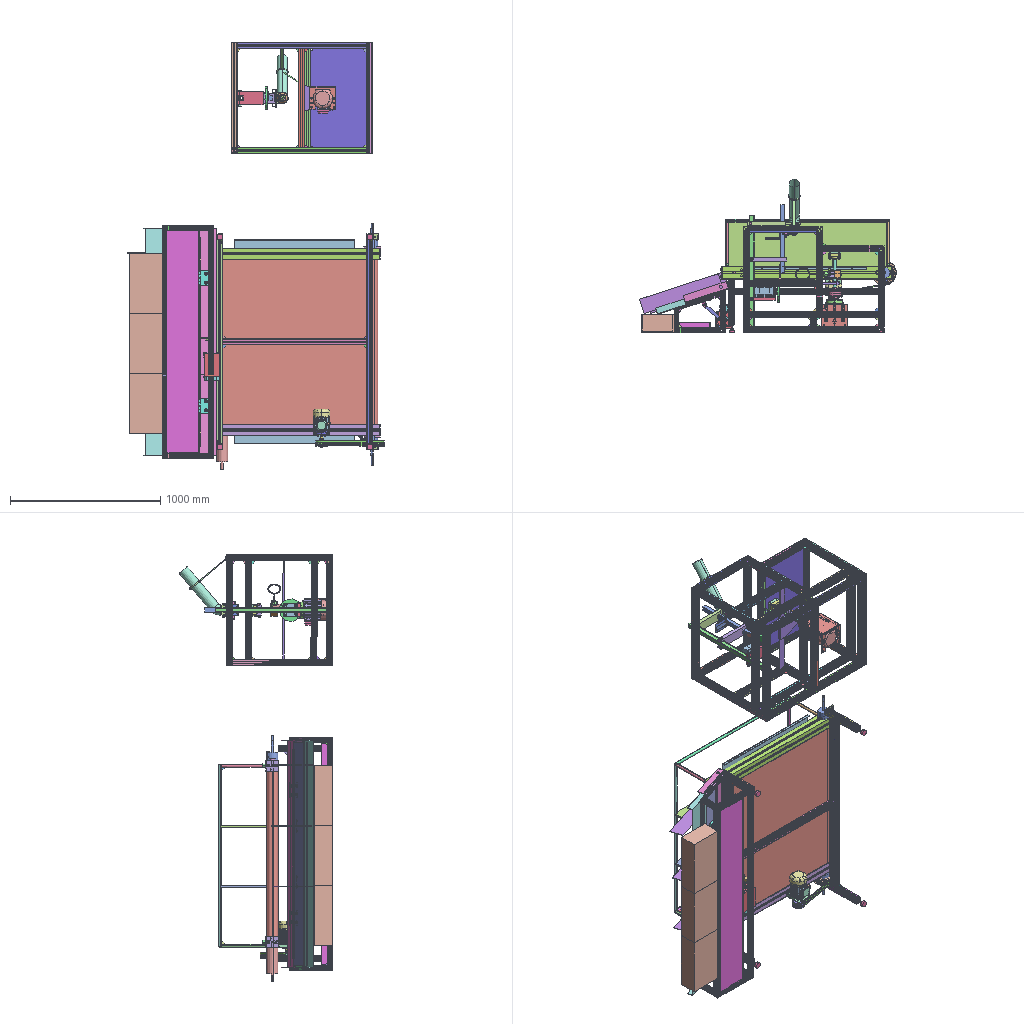Assembly | SolidWorks | 137 different items | 194 placed | box 1712 x 1025 x 2846 mm
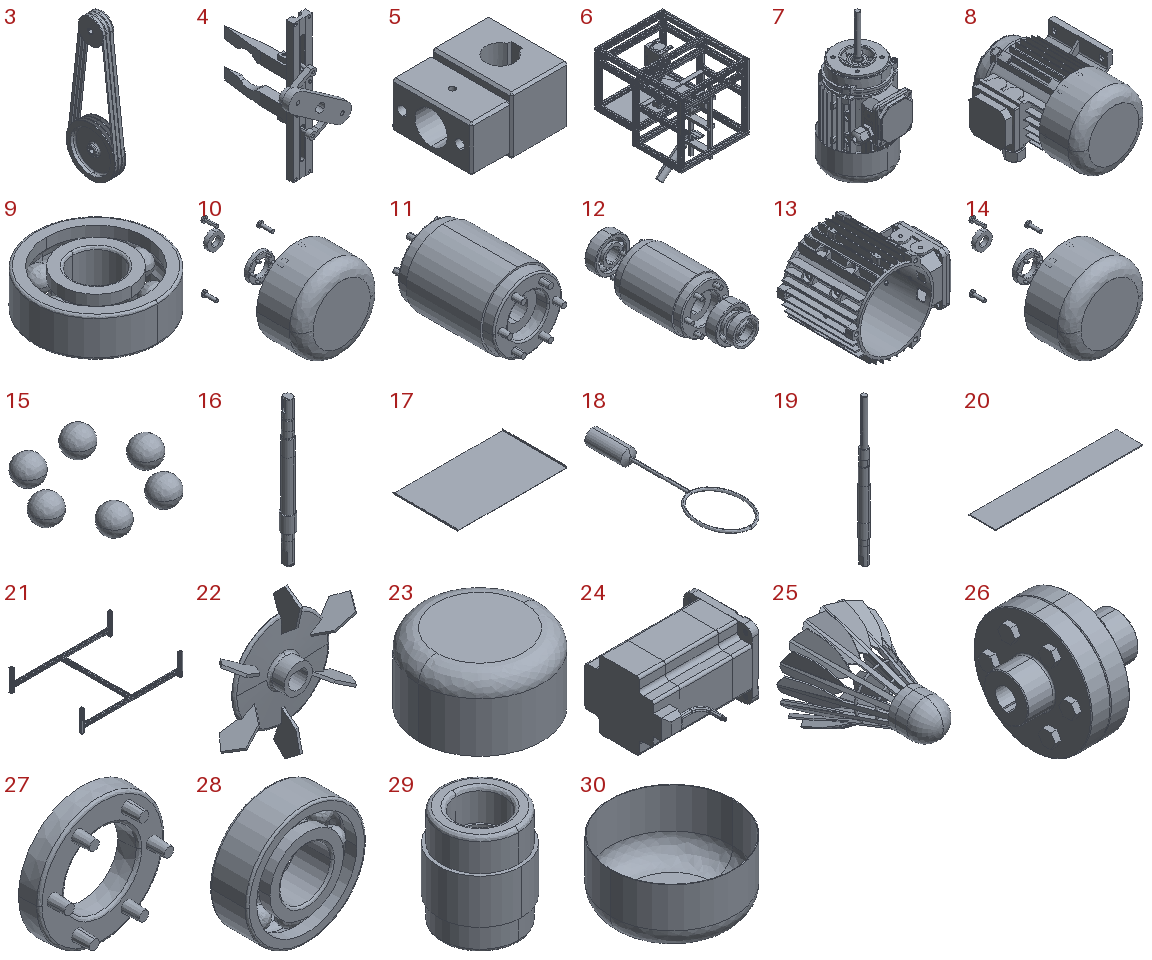Parts list (item | name | quantity | parent item | size | volume | features):
1 | 57BYG250C-57步进电机 | x1 | - | - | - | -
2 | (subassembly) | x1 | - | - | - | -
3 | (subassembly) | x1 | - | 38 x 164 x 475.5 mm | 628702 mm3 | features ReferencePattern 2, CompositeCurve 1, DerivedLPattern 1, InContextFeatHolder 1
4 | (subassembly) | x1 | in 6 | 54.684 x 83.216 x 120 mm | 23441 mm3 | features Cut 1, MirrorCompFeat 1
5 | (subassembly) | x1 | in 6 | 85 x 70 x 50 mm | 212005 mm3 | features Cut 1
6 | (subassembly) | x1 | - | - | 20823217 mm3 | features InContextFeatHolder 17, ReferencePattern 17, MirrorCompFeat 8, CompositeCurve 4, Cut 1, RefAxis 1
7 | (subassembly) | x1 | - | 115.663 x 132.2 x 251 mm | 733255 mm3 | -
8 | (subassembly) | x1 | in 6 | 169.5 x 250 x 139.906 mm | 665833 mm3 | -
9 | (subassembly) | x2 | in 12 | 32 x 32 x 10 mm | 4426 mm3 | -
10 | (subassembly) | x1 | in 14 | 136 x 218 x 136 mm | 125195 mm3 | -
11 | (subassembly) | x1 | in 12 | 47.5 x 74 x 47.5 mm | 93117 mm3 | -
12 | (subassembly) | x1 | in 7 | 47.5 x 132.5 x 47.5 mm | 103161 mm3 | -
13 | (subassembly) | x1 | in 7 | 130.2 x 96 x 112.64 mm | 107441 mm3 | -
14 | (subassembly) | x1 | in 8 | 136 x 218 x 136 mm | 125195 mm3 | -
15 | (subassembly) | x2 | in 9 | 28.05 x 25.096 x 5.88 mm | 678.568 mm3 | -
16 | - | x1 | in 8 | 20 x 20 x 234 mm | 48637 mm3 | features BaseBody 1
17 | - | x1 | - | 1360 x 800 x 20 mm | 3338438 mm3 | features EdgeFlange 1, FlatPattern 1, ICE 1, LPattern 1, MirrorPattern 1, SMBaseFlange 1, SheetMetal 1
18 | - | x1 | in 6 | 85 x 292.5 x 28 mm | 49744 mm3 | features ICE 2, RevCut 1, Sweep 1
19 | - | x1 | in 7 | - | - | features ICE 5, Chamfer 1, RefSurface 1, Revolution 1
20 | - | x3 | - | 550 x 100 x 3 mm | 165000 mm3 | features Extrusion 1
21 | - | x1 | - | 1440 x 1040 x 300 mm | 3739294 mm3 | features Gusset 12, 3DProfileFeature 1, WeldMemberFeat 1, WeldmentFeature 1
22 | - | x1 | in 8 | 103.191 x 21 x 118 mm | 16917 mm3 | features BaseBody 1
23 | - | x1 | in 10 | 136 x 136 x 75 mm | 33898 mm3 | features BaseBody 1
24 | - | x1 | in 6 | 165.5 x 124.49 x 85.5 mm | 823619 mm3 | features ICE 14, Fillet 3, CirPattern 2, CombineBodies 1, Extrusion 1, HoleWzd 1, LPattern 1, MoveCopyBody 1, RevCut 1, Sweep 1
25 | - | x1 | in 6 | 70.034 x 84.754 x 70.034 mm | 20525 mm3 | features CirPattern 3, ICE 3, CombineBodies 2, Revolution 2, Blend 1, PLine 1
26 | - | x1 | in 6 | 75 x 80 x 80 mm | 155086 mm3 | features ICE 16, Chamfer 6, Revolution 3, CirPattern 2, Fillet 2, RefAxis 1
27 | - | x2 | in 10, 11 | 45 x 13 x 45 mm | 7724 mm3 | features BaseBody 1
28 | - | x1 | in 8 | 35 x 11 x 35 mm | 5549 mm3 | features BaseBody 10
29 | - | x1 | in 7 | 90 x 90 x 108 mm | 413534 mm3 | features BaseBody 1
30 | - | x1 | in 7 | 114 x 114 x 57 mm | 16251 mm3 | features BaseBody 1
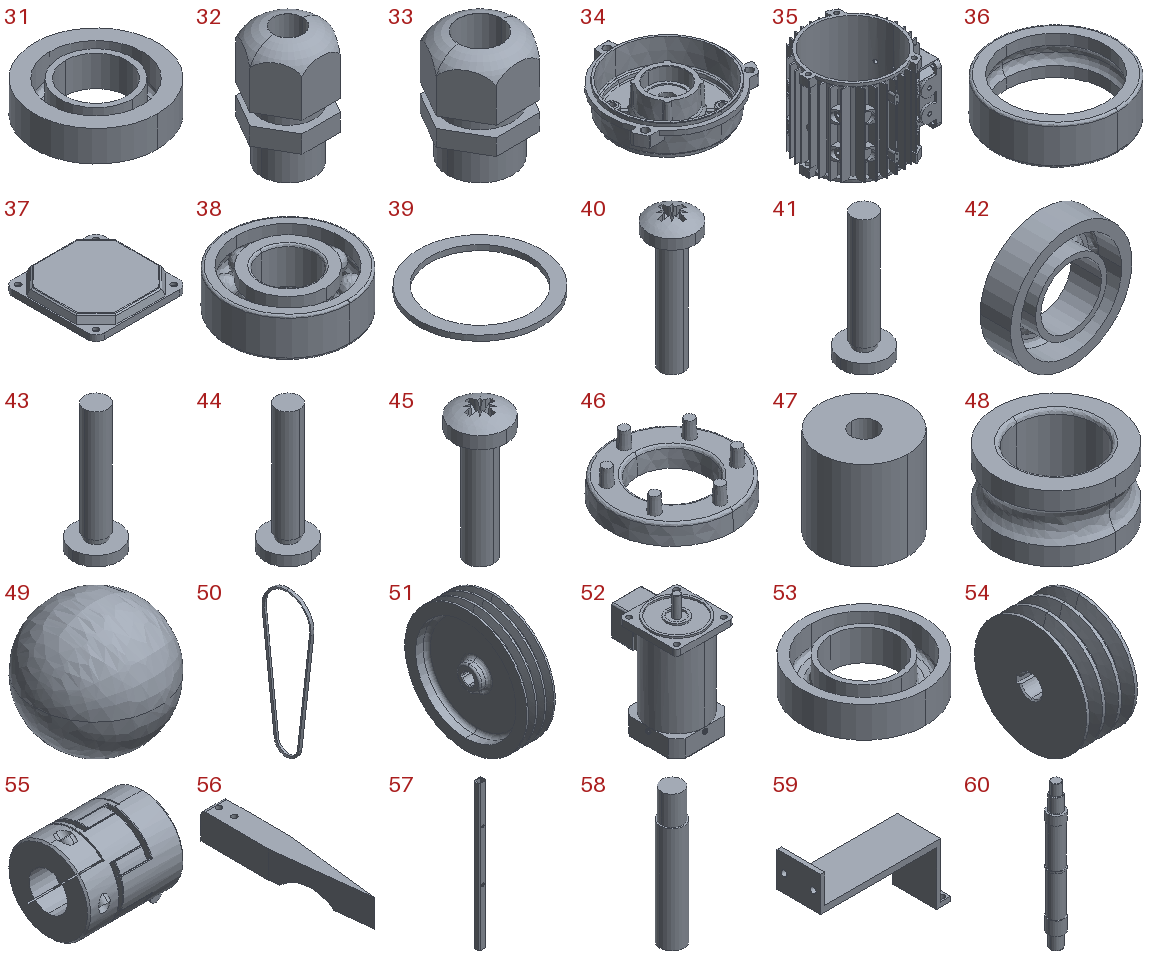31 | - | x1 | in 7 | 24 x 24 x 6 mm | 1505 mm3 | features BaseBody 1
32 | - | x1 | in 13 | 22.88 x 19.815 x 35.2 mm | 6256 mm3 | features BaseBody 1
33 | - | x1 | in 8 | 32.332 x 28 x 40 mm | 12162 mm3 | features BaseBody 1
34 | - | x1 | in 7 | 101.12 x 103.5 x 30 mm | 47636 mm3 | features BaseBody 1
35 | - | x1 | in 13 | 123 x 107.955 x 96 mm | 90735 mm3 | features BaseBody 5
36 | - | x2 | in 9 | 32 x 32 x 10 mm | 2470 mm3 | features BaseBody 1
37 | - | x1 | in 13 | 65 x 65 x 9.2 mm | 10449 mm3 | features BaseBody 1
38 | - | x1 | in 8 | 35 x 35 x 11 mm | 5549 mm3 | features BaseBody 10
39 | - | x1 | in 8 | 34.8 x 34.8 x 1.5 mm | 503.095 mm3 | features BaseBody 1
40 | - | x3 | in 7 | 8 x 8 x 23.025 mm | 359.622 mm3 | features BaseBody 1
41 | - | x1 | in 7 | 8 x 8 x 23.025 mm | 359.622 mm3 | features BaseBody 1
42 | - | x1 | in 12 | 24 x 6 x 24 mm | 1192 mm3 | features BaseBody 1
43 | - | x1 | in 7 | 8 x 8 x 23.025 mm | 359.622 mm3 | features BaseBody 1
44 | - | x1 | in 7 | 8 x 8 x 23.025 mm | 359.622 mm3 | features BaseBody 1
45 | - | x3 | in 10 | 9.5 x 9.5 x 23.612 mm | 579.898 mm3 | features BaseBody 1
46 | - | x1 | in 11 | 45 x 45 x 13 mm | 7724 mm3 | features BaseBody 1
47 | - | x1 | in 11 | 47.5 x 47.5 x 48 mm | 77670 mm3 | features BaseBody 1
48 | - | x2 | in 9 | 18.2 x 18.2 x 10 mm | 1277 mm3 | features BaseBody 1
49 | - | x12 | in 15 | - | 113.095 mm3 | features BaseBody 1
50 | - | x3 | in 3 | 10 x 160 x 471.5 mm | 52282 mm3 | features Sweep 1
51 | - | x1 | in 3 | 38 x 164 x 164 mm | 318015 mm3 | features Fillet 2, Chamfer 1, Cut 1, LPattern 1, RevCut 1, Revolution 1
52 | - | x1 | - | 106.313 x 147.157 x 215 mm | 1631430 mm3 | features BaseBody 1, HoleWzd 1
53 | - | x1 | in 10 | 28 x 28 x 7 mm | 1879 mm3 | features BaseBody 1
54 | - | x1 | in 3 | 38 x 84 x 84 mm | 153841 mm3 | features Chamfer 1, Cut 1, LPattern 1, RevCut 1, Revolution 1
55 | - | x1 | - | 35 x 31.403 x 31.299 mm | 17707 mm3 | features ICE 26, Fillet 5, CirPattern 4, Chamfer 2, Extrusion 2, Revolution 2
56 | - | x2 | in 4 | 8 x 60 x 10 mm | 3101 mm3 | features Cut 1, Extrusion 1, Fillet 1, ICE 1
57 | - | x1 | in 6 | 37 x 30 x 750 mm | 218758 mm3 | features ICE 2, Cut 1, Extrusion 1
58 | - | x2 | in 4 | 2.5 x 2.5 x 14 mm | 65.4 mm3 | features Extrusion 1, ICE 1
59 | - | x2 | in 6 | 45 x 15 x 30.5 mm | 1946 mm3 | features ICE 5, Extrusion 1
60 | - | x1 | in 6 | 28 x 28 x 254.001 mm | 113711 mm3 | features ICE 6, Fillet 3, Chamfer 2, Revolution 1
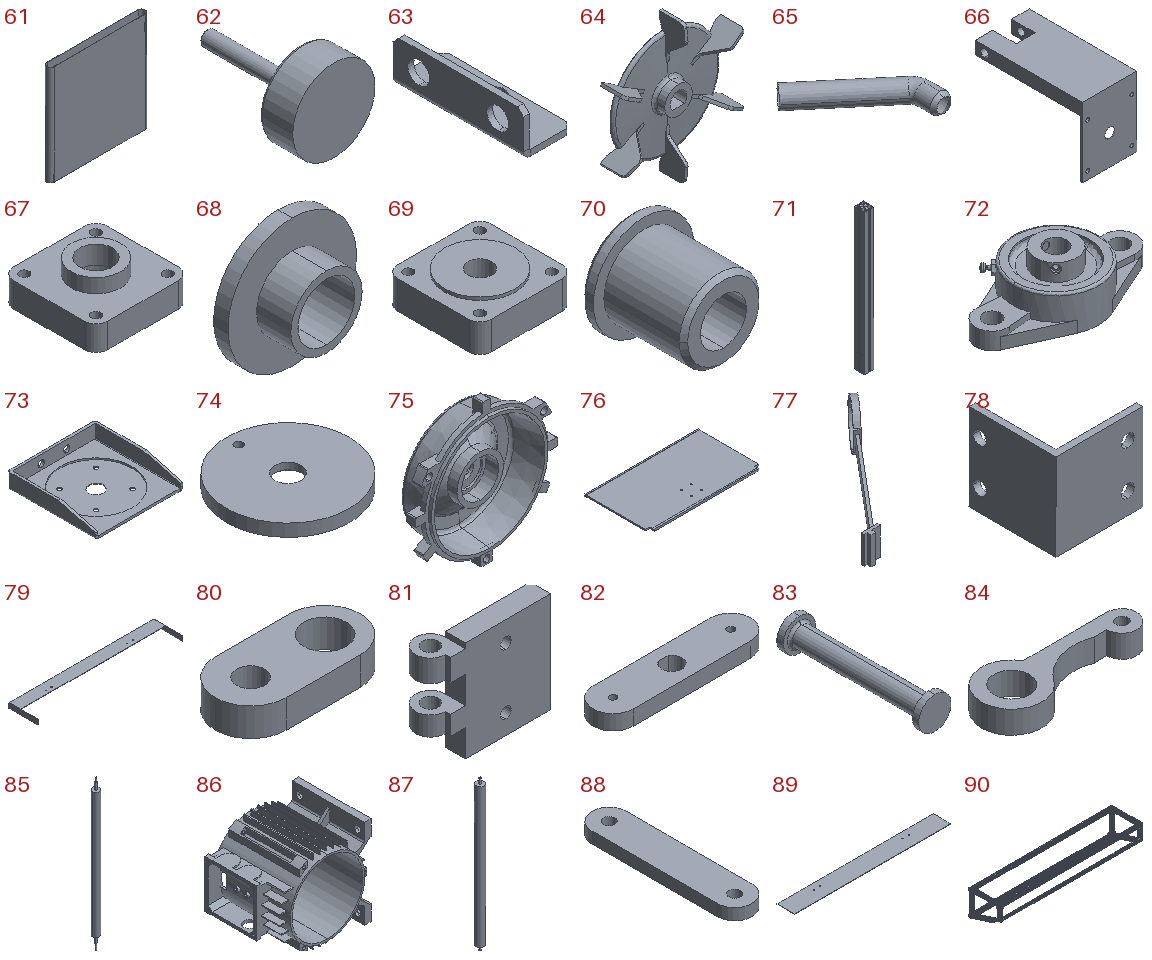61 | - | x1 | - | 1080 x 80 x 1100 mm | 4939097 mm3 | features ExtruThin 1
62 | - | x4 | - | 38.92 x 60 x 38.92 mm | 22752 mm3 | features Revolution 1
63 | - | x1 | - | 25 x 66 x 22 mm | 7707 mm3 | features HoleWzd 2, 3DProfileFeature 1, BreakCorner 1, EdgeFlange 1, FlatPattern 1, SMBaseFlange 1, SheetMetal 1
64 | - | x1 | in 7 | 85.87 x 18.15 x 98 mm | 14348 mm3 | features BaseBody 1
65 | - | x1 | in 6 | 325.613 x 346.787 x 70 mm | 94246 mm3 | features ICE 1, LoftedBend 1, Sweep 1, SweepCut 1
66 | - | x1 | in 6 | 85.5 x 169.57 x 110 mm | 284547 mm3 | features ICE 7, Cut 2, Extrusion 1, Fillet 1
67 | - | x1 | in 6 | 80 x 80 x 33 mm | 110292 mm3 | features Fillet 3, ICE 2, MirrorPattern 2, Extrusion 1, RevCut 1
68 | - | x1 | in 6 | 45 x 17 x 45 mm | 8502 mm3 | features ICE 1, Revolution 1
69 | - | x1 | in 6 | 80 x 80 x 26.5 mm | 139825 mm3 | features ICE 4, MirrorPattern 2, Extrusion 1, Fillet 1
70 | - | x1 | - | 24 x 22 x 24 mm | 4588 mm3 | features Chamfer 2, ICE 1, Revolution 1
71 | - | x3 | - | 76 x 85 x 1130 mm | 2230733 mm3 | features Cut 3, Extrusion 1, ICE 1
72 | - | x2 | - | 113 x 60 x 33.3 mm | 71709 mm3 | features Simplified 1
73 | - | x1 | - | 110 x 110 x 20 mm | 36896 mm3 | features ICE 5, MirrorPattern 2, Cut 1, EdgeFlange 1, Fillet 1, FlatPattern 1, SMBaseFlange 1, SheetMetal 1
74 | - | x1 | in 6 | 150 x 150 x 15 mm | 243715 mm3 | features Extrusion 1, ICE 1
75 | - | x1 | in 10 | 134 x 32.5 x 134 mm | 79781 mm3 | features BaseBody 1
76 | - | x1 | in 6 | 689 x 395 x 12 mm | 2213440 mm3 | features ICE 4, Cut 1, FlatPattern 1, SMBaseFlange 1, SheetMetal 1
77 | - | x1 | in 6 | 224.292 x 253.925 x 78 mm | 38659 mm3 | features ICE 7, MirrorPattern 2, BossThin 1, Extrusion 1
78 | - | x4 | - | 40 x 40 x 40 mm | 10463 mm3 | features ICE 2, FlatPattern 1, Gusset 1, SMBaseFlange 1, SheetMetal 1
79 | - | x1 | - | 1518 x 301 x 50 mm | 631038 mm3 | features ICE 6, EdgeFlange 2, FlatPattern 1, MirrorPattern 1, SMBaseFlange 1, SheetMetal 1
80 | - | x1 | - | 51.31 x 25 x 10 mm | 8934 mm3 | features Extrusion 1
81 | - | x4 | - | 115 x 35 x 100 mm | 190454 mm3 | features ICE 2, 3DProfileFeature 1, Chamfer 1, Extrusion 1, HoleWzd 1, MirrorPattern 1
82 | - | x1 | in 4 | 63.2 x 16 x 6 mm | 5359 mm3 | features ICE 3, Extrusion 1
83 | - | x2 | - | 25 x 110 x 25 mm | 22666 mm3 | features Fillet 1, Revolution 1
84 | - | x2 | in 4 | 31.031 x 12.062 x 4.5 mm | 635.986 mm3 | features Extrusion 1
85 | - | x1 | - | 76 x 76 x 1615 mm | 6202615 mm3 | features ICE 5, MirrorPattern 2, Extrusion 1
86 | - | x1 | in 8 | 147 x 119 x 138 mm | 264142 mm3 | features BaseBody 3
87 | - | x1 | - | 76 x 76 x 1450 mm | 6144327 mm3 | features Extrusion 1, ICE 1, MirrorPattern 1
88 | - | x1 | in 6 | 30 x 140 x 10 mm | 38498 mm3 | features Extrusion 1
89 | - | x1 | - | 1500 x 170 x 3 mm | 764058 mm3 | features ICE 2, Extrusion 1, MirrorPattern 1
90 | - | x1 | - | 1548 x 337.768 x 285.646 mm | 2440117 mm3 | features Gusset 16, WeldCornerFeat 2, 3DProfileFeature 1, ICE 1, WeldMemberFeat 1, WeldmentFeature 1
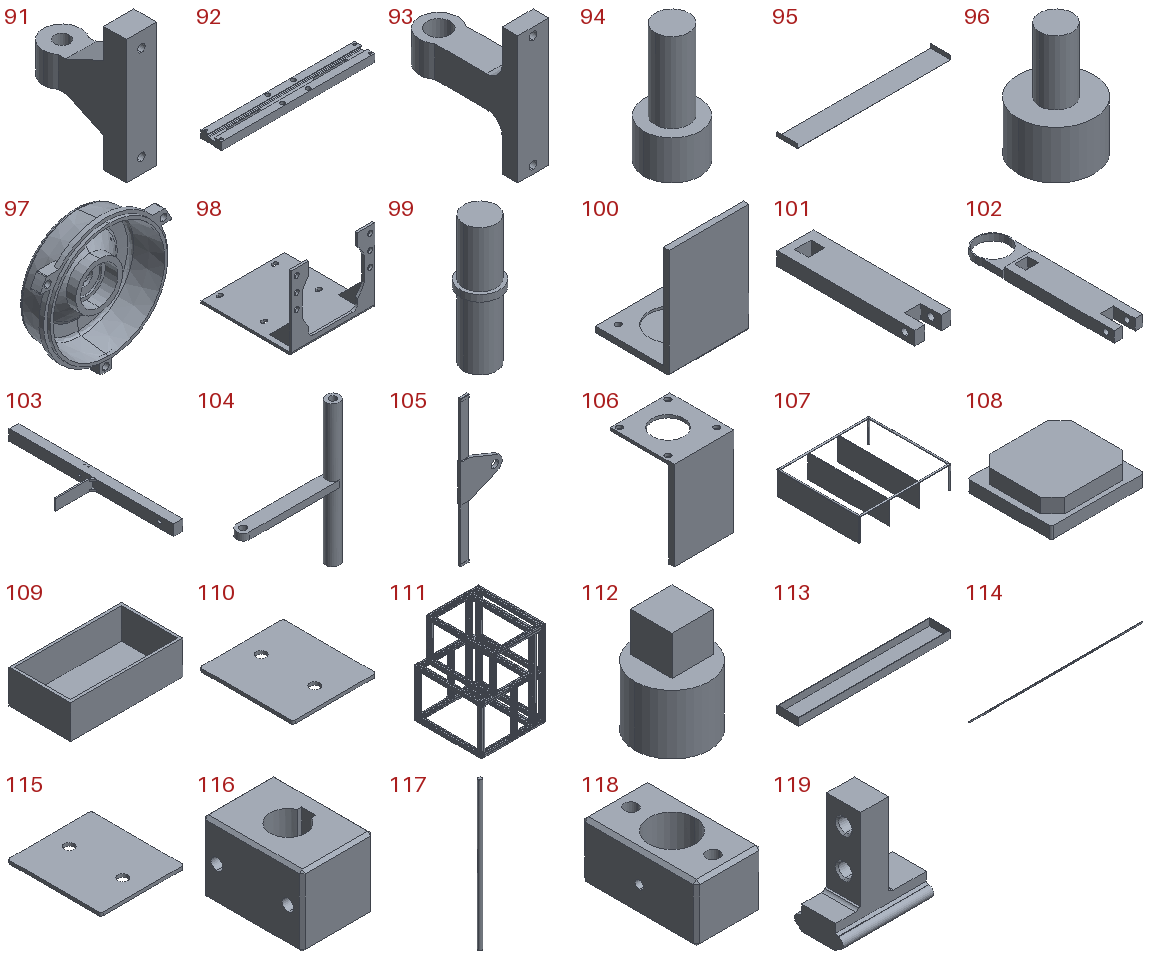91 | - | x2 | - | 25 x 65 x 82.337 mm | 48790 mm3 | features ICE 2, 3DProfileFeature 1, Extrusion 1, HoleWzd 1, MirrorPattern 1
92 | - | x1 | in 4 | 120 x 16.4 x 6 mm | 8918 mm3 | features ICE 4, Cut 2, Extrusion 1
93 | - | x1 | - | 25 x 73.5 x 82.337 mm | 39218 mm3 | features ICE 2, 3DProfileFeature 1, Extrusion 1, HoleWzd 1, MirrorPattern 1
94 | - | x4 | in 4 | 3.3 x 3.3 x 7 mm | 34.437 mm3 | features Extrusion 1, ICE 1
95 | - | x1 | - | 1518 x 200 x 41 mm | 351600 mm3 | features Extrusion 1, ICE 1, MirrorPattern 1
96 | - | x2 | in 4 | 7.08 x 7.08 x 10.5 mm | 221.865 mm3 | features Extrusion 1, ICE 1
97 | - | x1 | in 8 | 122.449 x 32.5 x 125 mm | 76079 mm3 | features BaseBody 1
98 | - | x1 | in 6 | 170 x 185 x 150 mm | 223380 mm3 | features Gusset 2, ICE 2, 3DProfileFeature 1, Cut 1, EdgeFlange 1, Fillet 1, FlatPattern 1, HoleWzd 1, LPattern 1, MirrorPattern 1, SMBaseFlange 1, SheetMetal 1
99 | - | x1 | - | 18 x 18 x 58.5 mm | 10571 mm3 | features ICE 4, Extrusion 1
100 | - | x1 | in 6 | 70 x 65 x 95 mm | 51093 mm3 | features ICE 4, Fillet 2, Extrusion 1
101 | - | x1 | in 6 | 66 x 252 x 25 mm | 365157 mm3 | features ICE 2, 3DProfileFeature 1, Extrusion 1, HoleWzd 1, MirrorPattern 1
102 | - | x1 | in 6 | 77 x 350 x 25 mm | 393296 mm3 | features ICE 3, 3DProfileFeature 1, BossThin 1, Extrusion 1, Fillet 1, HoleWzd 1, MirrorPattern 1
103 | - | x1 | in 6 | 127.6 x 455 x 30 mm | 350644 mm3 | features ICE 3, Cut 2, Gusset 2, Extrusion 1, Fillet 1, WeldmentFeature 1
104 | - | x1 | - | 153.27 x 20 x 210 mm | 75349 mm3 | features ICE 3, Extrusion 1
105 | - | x1 | in 6 | 195.363 x 15 x 689 mm | 515152 mm3 | features ICE 6, Cut 1, Extrusion 1, Fillet 1, MirrorPattern 1
106 | - | x1 | - | 104 x 111.35 x 155 mm | 184852 mm3 | features ICE 2, Cut 1, Extrusion 1
107 | - | x1 | - | 1220 x 1093 x 315 mm | 10289928 mm3 | features 3DProfileFeature 2, Gusset 2, ExtruThin 1, WeldMemberFeat 1, WeldmentFeature 1
108 | - | x1 | in 8 | 80 x 72 x 22.5 mm | 111066 mm3 | features BaseBody 1
109 | - | x3 | - | 400 x 220 x 120 mm | 2200000 mm3 | features ExtruThin 1, ICE 1
110 | - | x3 | - | 76 x 85 x 3 mm | 18988 mm3 | features 3DProfileFeature 1, BreakCorner 1, FlatPattern 1, HoleWzd 1, MirrorPattern 1, SMBaseFlange 1, SheetMetal 1
111 | - | x1 | in 6 | 710 x 740 x 940 mm | 13346317 mm3 | features Gusset 71, WeldCornerFeat 9, 3DProfileFeature 1, WeldMemberFeat 1, WeldmentFeature 1
112 | - | x4 | - | 25 x 25 x 34.87 mm | 7814 mm3 | features ICE 3, Chamfer 1, Extrusion 1
113 | - | x1 | - | 1480 x 210 x 70 mm | 2646000 mm3 | features ExtruThin 1, ICE 1
114 | - | x2 | - | 1390 x 5 x 10 mm | 29876 mm3 | features ICE 4, ExtruThin 1, MirrorPattern 1
115 | - | x3 | - | 76 x 85 x 3 mm | 18988 mm3 | features 3DProfileFeature 1, BreakCorner 1, FlatPattern 1, HoleWzd 1, ICE 1, MirrorPattern 1, SMBaseFlange 1, SheetMetal 1
116 | - | x1 | in 5 | 50 x 70 x 50 mm | 143509 mm3 | features ICE 3, Chamfer 1, Extrusion 1, MirrorPattern 1
117 | - | x1 | - | 10 x 10 x 400 mm | 31416 mm3 | features Extrusion 1
118 | - | x1 | in 5 | 40 x 70 x 35 mm | 71575 mm3 | features ICE 2, MirrorPattern 2, 3DProfileFeature 1, Chamfer 1, Extrusion 1, HoleWzd 1
119 | - | x2 | in 4 | 13.3 x 7.2 x 16 mm | 492.464 mm3 | features ICE 5, Chamfer 3, HoleWzd 2, Cut 1, Extrusion 1
120 | circlips for shaft--type a large gb | x1 | - | - | - | -
121 | cross recessed cheese head screws type a gb | x1 | - | - | - | -
122 | deep groove ball bearings gb | x1 | - | - | - | -
123 | hex head bolts-full thread grade c gb | x1 | - | - | - | -
124 | hex lobular socket head cap screws-4.8 gb | x1 | - | - | - | -
125 | hex nut-fine pitch-style washer-grade ab gb | x1 | - | - | - | -
126 | hex nuts 1-fine pitch-grades ab gb | x1 | - | - | - | -
127 | hex nuts, style 1-grades ab gb | x1 | - | - | - | -
128 | hex nuts-style normal-grades ab gb | x1 | - | - | - | -
129 | hexagon head bolts-full thread gb | x1 | - | - | - | -
130 | hexagon nuts grade c gb | x1 | - | - | - | -
131 | parallel pins hardening steel gb | x1 | - | - | - | -
132 | parallel pins unhardening steel gb | x1 | - | - | - | -
133 | plain parallel keys | x1 | - | - | - | -
134 | plain washers-s series-grade a gb | x1 | - | - | - | -
135 | rubber dust seals type a gb | x1 | - | - | - | -
136 | taper keys for general use gb | x1 | - | - | - | -
137 | thrust ball bearings gb | x1 | - | - | - | -
Mates (type | each side: item.copy, entity, surface, feature):
In the top assembly
Symmetric | 71.1 face plane | 71.1 face plane | assembly plane
Concentric | 85.1 face cylinder Boss-Extrude 2 | 72.1 face cylinder 已转换1
Width | 71.1 face plane | 71.1 face plane | 72.1 face plane 已转换1 | 72.1 face plane 已转换1
Coincident | 71.1 face plane | 72.1 face plane 已转换1
Coincident | 71.1 face plane | 110.1 face plane Base-Flange 1 | 2 times
Width | 110.1 face plane Base-Flange 1 | 110.1 face plane Base-Flange 1 | 71.1 face plane | 71.1 face plane
Width | 71.1 face plane | 71.1 face plane | 115.1 face plane Base-Flange 1 | 115.1 face plane Base-Flange 1
Coincident | 71.1 face plane | 115.1 face plane Base-Flange 1 | 2 times
Concentric | 85.1 face cylinder Mirror 1 | 72.2 face cylinder 已转换1
Coincident | 71.2 face plane | 72.2 face plane 已转换1
Coincident | 17.1 plane | assembly plane
Width | 71.2 face plane | 71.1 face plane | 17.1 face plane Mirror 1 | 17.1 face plane Edge-Flange 1
Width | 110.1 face plane Base-Flange 1 | 115.1 face plane Base-Flange 1 | 17.1 face plane Base-Flange 1 | 17.1 face plane Base-Flange 1
Symmetric | 21.1 face plane Aluminium Profile 40 X 40GF X R0.5(3) | 21.1 face plane Aluminium Profile 40 X 40GF X R0.5(3) | assembly plane
Coincident | 71.1 face plane | 21.1 face plane Aluminium Profile 40 X 40GF X R0.5(3)
Width | 71.2 face plane | 71.1 face plane | 21.1 face plane Aluminium Profile 40 X 40GF X R0.5(3) | 21.1 face plane Aluminium Profile 40 X 40GF X R0.5(3)
Width | 71.2 face plane | 71.2 face plane | 63.1 face plane Edge-Flange 1 | 63.1 face plane Edge-Flange 1
Coincident | 71.2 face plane | 63.1 face plane Edge-Flange 1
Parallel | 71.2 face plane | 72.2 face plane 已转换1
Coincident | 71.2 face plane | 73.1 face plane Base-Flange 1 | 2 times
Concentric | 85.1 face cylinder Boss-Extrude 1 | 61.1 face cylinder Extrude-薄壁1
Coincident | 17.1 face plane Base-Flange 1 | 61.1 face plane Extrude-薄壁1
Coincident | 71.2 face plane | 61.1 face plane Extrude-薄壁1
Coincident | 71.1 face plane | 61.1 face plane Extrude-薄壁1
Width | 71.1 face plane | 71.2 face plane | 85.1 face plane Boss-Extrude 1 | 85.1 face plane Boss-Extrude 1
Concentric | 87.1 face cylinder Boss-Extrude 1 | 61.1 face cylinder Extrude-薄壁1
Coincident | 21.1 face plane Aluminium Profile 40 X 40GF X R0.5(3) | 78.1 face plane Base-Flange 1 | 2 times
Coincident | 71.1 face plane | 78.1 face plane Base-Flange 1
Concentric | 81.1 face cylinder Cut-Extrude 1 | 83.1 face cylinder Revolve 2
Width | 83.1 face plane Revolve 2 | 83.1 face plane Revolve 2 | 81.2 face plane Boss-Extrude 2 | 81.2 face plane Boss-Extrude 2
Concentric | 81.2 face cylinder Cut-Extrude 1 | 83.1 face cylinder Revolve 2
Width | 81.2 face plane Boss-Extrude 2 | 81.2 face plane Boss-Extrude 2 | 81.1 face plane Boss-Extrude 2 | 81.1 face plane Boss-Extrude 2
Width | 90.1 face plane Aluminium Profile 30X 30G X R1.5(1) | 90.1 face plane Aluminium Profile 30X 30G X R1.5(1) | 21.1 face plane Aluminium Profile 40 X 40GF X R0.5(3) | 21.1 face plane Aluminium Profile 40 X 40GF X R0.5(3)
Parallel | 62.1 face plane Revolve 1 | 90.1 face plane Aluminium Profile 30X 30G X R1.5(1)
DistanceDim | 90.1 face plane Aluminium Profile 30X 30G X R1.5(1) | 21.1 face plane Aluminium Profile 40 X 40GF X R0.5(3)
Coincident | 62.1 face plane Revolve 1 | 90.1 face plane Aluminium Profile 30X 30G X R1.5(1)
Concentric | 21.1 face cylinder Aluminium Profile 40 X 40GF X R0.5(3) | 62.2 face cylinder Revolve 1
Concentric | 81.2 face cylinder M10 六角头Bolt的柱形沉头Hole 1 | 89.1 face cylinder
Concentric | 81.2 face cylinder Mirror 1 | 89.1 face cylinder
Coincident | 81.2 face plane Boss-Extrude 2 | 89.1 face plane
Coincident | 89.1 face plane | 91.1 face plane Boss-Extrude 3
Parallel | 90.1 face plane Aluminium Profile 30X 30G X R1.5(1) | 95.1 face plane Boss-Extrude 1
DistanceDim | 95.1 face plane Boss-Extrude 1 | 90.1 face plane Cut-Extrude 1
Coincident | 90.1 face plane Cut-Extrude 1 | 95.1 face plane Boss-Extrude 1
Concentric | 89.1 face cylinder Cut-Extrude 5 | 91.1 face cylinder Mirror 1
Concentric | 89.1 face cylinder Cut-Extrude 5 | 91.1 face cylinder M6 Tapped Hole 1
Coincident | 90.1 face plane Aluminium Profile 30X 30G X R1.5(1) | 93.1 face plane Boss-Extrude 3 | 2 times
Concentric | 81.3 face cylinder Cut-Extrude 1 | 83.2 face cylinder Revolve 2
Width | 81.4 face plane Cut-Extrude 8 | 81.3 face plane Cut-Extrude 8 | 83.2 face plane Revolve 2 | 83.2 face plane Revolve 2
Concentric | 85.1 face cylinder Mirror 1 | 51.1 face cylinder Revolve 1
Coincident | 72.2 face plane 已转换1 | 51.1 face plane Revolve 1
Coincident | 73.1 face plane Base-Flange 1 | 70.1 edge
Parallel | 61.1 face plane Extrude-薄壁1 | 107.1 face plane Extrude-薄壁2
Parallel | 115.2 face plane Base-Flange 1 | 107.1 face plane Extrude-薄壁2
Width | 115.2 face plane Base-Flange 1 | 110.2 face plane Base-Flange 1 | 107.1 face plane Extrude-薄壁2 | 107.1 face plane Extrude-薄壁2
Parallel | 90.1 face plane Aluminium Profile 30X 30G X R1.5(1) | 109.1 face plane Extrude-薄壁1
Coincident | 90.1 face plane Aluminium Profile 30X 30G X R1.5(1) | 109.2 face plane Extrude-薄壁1 | 2 times
Concentric | 91.1 face cylinder Boss-Extrude 1 | 117.1 face cylinder Boss-Extrude 1
Width | 117.1 face plane Boss-Extrude 1 | 117.1 face plane Boss-Extrude 1 | 91.1 face plane Boss-Extrude 1 | 91.2 face plane Boss-Extrude 1
Width | 90.1 face plane Aluminium Profile 30X 30G X R1.5(1) | 90.1 face plane Aluminium Profile 30X 30G X R1.5(1) | 93.1 face plane Boss-Extrude 3 | 93.1 face plane Boss-Extrude 3
Concentric | 80.1 face cylinder Boss-Extrude 1 | 93.1 face cylinder Boss-Extrude 1 | 2 times
Concentric | 104.1 face cylinder Cut-Extrude 1 | 117.1 face cylinder Boss-Extrude 1
Concentric | 80.1 face cylinder Boss-Extrude 1 | 104.1 face cylinder Boss-Extrude 1
Concentric | 55.1 face cylinder Cut-Extrude 7 | 99.1 face cylinder Boss-Extrude 1
Coincident | 93.1 face plane Boss-Extrude 1 | 99.1 face plane Boss-Extrude 2
Coincident | 80.1 face plane Boss-Extrude 1 | 104.1 face plane Boss-Extrude 1
Coincident | 80.1 face plane Boss-Extrude 1 | 93.1 face plane Boss-Extrude 1
Concentric | 107.1 face cylinder 圆管 20X1.2(1) | 112.1 face cylinder Cut-Extrude 1
Coincident | 71.1 face plane | 112.1 face plane Boss-Extrude 3
Coincident | 71.1 face plane | 112.1 face plane Boss-Extrude 2
Coincident | 107.1 face plane 圆管 20X1.2(1) | 112.1 face plane Cut-Extrude 1
Concentric | 107.1 face cylinder 圆管 20X1.2(1) | 112.2 face cylinder Cut-Extrude 1
Parallel | 71.1 face plane | 112.2 face plane Boss-Extrude 3
Coincident | 71.1 face plane | 112.2 face plane Boss-Extrude 3
Concentric | 87.1 face cylinder Mirror 1 | 71.3 face cylinder Cut-Extrude 5
Concentric | 80.1 face cylinder Boss-Extrude 1 | 99.1 face cylinder Boss-Extrude 1
Concentric | 52.1 face cylinder 输入1 | 99.1 face cylinder Boss-Extrude 1
DistanceDim | 52.1 face plane 输入1 | 99.1 face plane Boss-Extrude 1
Parallel | 90.1 face plane Aluminium Profile 30X 30G X R1.5(1) | 52.1 face plane 输入1
Concentric | 99.1 face cylinder Boss-Extrude 1 | 106.1 face cylinder Cut-Extrude 4
Coincident | 52.1 face plane 输入1 | 106.1 face plane Boss-Extrude 1
Parallel | 52.1 face plane 输入1 | 106.1 face plane Boss-Extrude 1
Coincident | 90.1 face plane Aluminium Profile 30X 30G X R1.5(1) | 109.1 face plane Extrude-薄壁1
Coincident | 90.1 face plane Aluminium Profile 30X 30G X R1.5(1) | 109.3 face plane Extrude-薄壁1
Parallel | 90.1 face plane Aluminium Profile 30X 30G X R1.5(1) | 113.1 face plane Boss-Extrude 1
Width | 90.1 face plane Aluminium Profile 30X 30G X R1.5(1) | 90.1 face plane Aluminium Profile 30X 30G X R1.5(1) | 113.1 face plane Extrude-薄壁1 | 113.1 face plane Extrude-薄壁1
Coincident | 107.1 face plane Extrude-薄壁2 | 109.2 face plane Extrude-薄壁1
Coincident | 107.1 face plane Extrude-薄壁2 | 109.3 face plane Extrude-薄壁1
Coincident | 107.1 face plane Extrude-薄壁2 | 109.1 face plane Extrude-薄壁1
Coincident | 87.1 face plane Boss-Extrude 1 | 71.1 face plane
Concentric | 54.1 face cylinder Revolve 1 | 70.1 face cylinder Revolve 1
Concentric | 70.1 face cylinder Revolve 1 | 19.1 face cylinder Boss-Extrude 2
Concentric | 73.1 face cylinder Cut-Extrude 4 | 19.1 face cylinder Boss-Extrude 2
Parallel | 73.1 face plane Base-Flange 1 | 37.1 face plane 输入1
Coincident | 73.1 face plane Cut-Extrude 6 | 34.1 face plane 输入1
Coincident | 90.1 face plane Aluminium Profile 30X 30G X R1.5(1) | 113.1 face plane Extrude-薄壁1 | 2 times
Width | 89.1 face plane | 89.1 face plane | 114.1 face plane Extrude-薄壁1 | 114.1 face plane Extrude-薄壁1
Coincident | 89.1 face plane | 114.1 face plane Boss-Extrude 1
Coincident | 89.1 face plane | 114.1 face plane Extrude-薄壁1
Concentric | 79.1 face cylinder Cut-Extrude 3 | 81.1 face cylinder Mirror 1
Coincident | 79.1 face plane Base-Flange 1 | 81.1 face plane Boss-Extrude 2
Width | 71.1 face plane | 71.2 face plane | 79.1 face plane Edge-Flange 2 | 79.1 face plane Edge-Flange 1
Parallel | 79.1 face plane Base-Flange 1 | 90.1 face plane Aluminium Profile 30X 30G X R1.5(1)
Coincident | 79.1 face plane Base-Flange 1 | 90.1 face plane Aluminium Profile 30X 30G X R1.5(1)
DistanceDim | 79.1 vertex | 90.1 face plane 剪裁/延伸3
Width | 79.1 face plane Edge-Flange 2 | 79.1 face plane Edge-Flange 1 | 95.1 face plane Boss-Extrude 1 | 95.1 face plane Boss-Extrude 1
Width | 79.1 face plane Edge-Flange 2 | 79.1 face plane Edge-Flange 1 | 114.2 face plane Extrude-薄壁1 | 114.2 face plane Extrude-薄壁1
Coincident | 79.1 face plane Cut-Extrude 2 | 114.2 face plane Boss-Extrude 1
Coincident | 79.1 face plane Base-Flange 1 | 114.2 face plane Extrude-薄壁1
Coincident | 109.1 face plane Extrude-薄壁1 | 109.3 face plane Extrude-薄壁1
Parallel | 90.1 face cylinder Aluminium Profile 30X 30G X R1.5(1) | 20.1 edge
Parallel | 20.1 face plane Boss-Extrude 1 | 20.2 face plane Boss-Extrude 1
Parallel | 90.1 edge | 20.3 edge
Parallel | 90.1 edge | 111.1 edge
In subassembly 6
Concentric | 74.1 face cylinder Boss-Extrude 1 | 88.1 face cylinder Boss-Extrude 1
Coincident | 74.1 face plane Boss-Extrude 1 | 88.1 face plane Boss-Extrude 1
Concentric | 88.1 face cylinder Boss-Extrude 1 | 103.1 face cylinder Cut-Extrude 1
Coincident | 88.1 face plane Boss-Extrude 1 | 103.1 face plane Boss-Extrude 2
Concentric | 60.1 face cylinder Revolve 1 | 116.1 face cylinder
Concentric | 118.1 face cylinder Cut-Extrude 1 | 18.1 face cylinder Boss-Extrude 2
Coincident | 116.1 face plane Cut-Extrude 1 | 18.1 face plane Boss-Extrude 2
PlanarAngleDim | 18.1 plane | 5.1 plane
Concentric | 60.1 face cylinder Revolve 1 | 26.1 face cylinder Cut-Extrude 6
Coincident | 60.1 face plane Revolve 1 | 26.1 face plane Revolve 2
DistanceDim | 103.1 face plane Boss-Extrude 2 | 82.1 face plane Boss-Extrude 1
Width | 111.2 face plane Aluminium Profile 40 X 40GF X R0.5(1) | 111.2 face plane Aluminium Profile 40 X 40GF X R0.5(1) | 57.1 face plane | 57.1 face plane
Concentric | 57.1 face cylinder | 66.1 face cylinder Cut-Extrude 2
Coincident | 57.1 face plane | 66.1 face plane Cut-Extrude 1
Parallel | 111.2 face plane Aluminium Profile 40 X 40GF X R0.5(1) | 66.1 face plane Boss-Extrude 1
Coincident | 111.2 face plane Aluminium Profile 40 X 40GF X R0.5(1) | 57.1 face plane
Coincident | 103.1 plane | 57.1 plane
Coincident | 101.1 face plane Boss-Extrude 1 | 57.1 face plane
Concentric | 101.1 face cylinder M14 Tapped Hole 1 | 57.1 face cylinder
Coincident | 66.1 face plane Boss-Extrude 1 | 24.1 face plane Boss-Extrude 1
Concentric | 74.1 face cylinder Boss-Extrude 1 | 24.1 face cylinder Boss-Extrude 3
Concentric | 26.1 face cylinder Cut-Extrude 15 | 16.1 face cylinder 输入1
Parallel | 111.2 face plane Aluminium Profile 40 X 40GF X R0.5(1) | 86.1 face plane 输入3
Coincident | 86.1 face plane 输入3 | 98.1 face plane Base-Flange 1
Width | 98.1 face plane Base-Flange 1 | 98.1 face plane Base-Flange 1 | 86.1 face plane 输入3 | 86.1 face plane 输入3
Concentric | 65.1 face cylinder Sweep 4 | 77.1 face cylinder Extrude-薄壁2
Concentric | 65.1 face cylinder Cut-Sweep 1 | 6.1 axis
Coincident | 74.1 face plane Boss-Extrude 1 | 24.1 face plane Boss-Extrude 3
Coincident | 111.2 edge | 76.1 face plane Base-Flange 1
Width | 24.1 face plane Boss-Extrude 1 | 24.1 face plane Boss-Extrude 1 | 66.1 face plane Boss-Extrude 1 | 66.1 face plane Boss-Extrude 1
Parallel | 103.1 face plane Boss-Extrude 4 | 102.1 face plane Boss-Extrude 1
DistanceDim | 102.1 face plane Boss-Extrude 1 | 57.1 face plane
Coincident | 92.1 face plane Boss-Extrude 1 | 59.1 face plane Boss-Extrude 1
Parallel | 92.1 face plane Boss-Extrude 1 | 59.1 face plane Boss-Extrude 1
Coincident | 92.1 face plane Boss-Extrude 1 | 59.1 face plane Boss-Extrude 2
Width | 92.1 face plane Boss-Extrude 1 | 92.1 face plane Boss-Extrude 1 | 59.1 face plane Boss-Extrude 1 | 59.1 face plane Boss-Extrude 1
Coincident | 66.1 face plane Boss-Extrude 2 | 24.1 face plane Boss-Extrude 1
Coincident | 111.2 face plane Aluminium Profile 40 X 40GF X R0.5(1) | 77.1 face plane Boss-Extrude 1
Coincident | 111.2 face plane Aluminium Profile 40 X 40GF X R0.5(1) | 77.1 face plane Cut-Extrude 4
Concentric | 67.1 face cylinder Mirror 2 | 69.1 face cylinder Mirror 2
Concentric | 67.1 face cylinder Cut-Extrude 1 | 69.1 face cylinder Cut-Extrude 1
Coincident | 67.1 face plane Boss-Extrude 1 | 69.1 face plane Boss-Extrude 1
Parallel | 69.1 face plane Boss-Extrude 1 | 111.2 face plane Aluminium Profile 40 X 40GF X R0.5(1)
Coincident | 111.2 face plane Aluminium Profile 40 X 40GF X R0.5(1) | 76.1 face plane Base-Flange 1 | 4 times
Coincident | 111.2 face plane Aluminium Profile 40 X 40GF X R0.5(1) | 76.1 face plane Boss-Extrude 1
Coincident | 69.1 face plane Boss-Extrude 1 | 76.1 face plane Base-Flange 1
Parallel | 103.1 face plane Boss-Extrude 2 | 101.1 face plane Boss-Extrude 1
Width | 102.1 face plane Boss-Extrude 1 | 102.1 face plane Boss-Extrude 1 | 57.1 face plane | 57.1 face plane
Coincident | 103.1 face plane Boss-Extrude 2 | 102.1 face plane Cut-Extrude 1
Coincident | 111.2 face plane Aluminium Profile 40 X 40GF X R0.5(1) | 105.1 face plane Boss-Extrude 1 | 2 times
Coincident | 111.2 face plane Aluminium Profile 40 X 40GF X R0.5(1) | 105.1 face plane Boss-Extrude 10
Concentric | 60.1 face cylinder Revolve 1 | 67.1 face cylinder Cut-Revolve 1
Coincident | 60.1 face plane Boss-Extrude 2 | 116.1 face plane
Coincident | 60.1 face plane Revolve 1 | 67.1 face plane Cut-Revolve 1
In subassembly 5
Concentric | 116.2 face cylinder | 118.2 face cylinder Cut-Extrude 3
In subassembly 4
Coincident | 82.2 face plane Boss-Extrude 1 | 84.1 face plane Boss-Extrude 1
Concentric | 82.2 face cylinder Cut-Extrude 1 | 84.1 face cylinder Boss-Extrude 1
Concentric | 84.1 face cylinder Boss-Extrude 1 | 58.1 face cylinder Boss-Extrude 1
Coincident | 84.1 face plane Boss-Extrude 1 | 58.1 face plane Boss-Extrude 1
Concentric | 58.1 face cylinder Boss-Extrude 1 | 119.1 face cylinder Cut-Extrude 10
Coincident | 58.1 face plane Boss-Extrude 1 | 119.1 face plane Cut-Extrude 10
DistanceDim | 92.2 face plane Cut-Extrude 5 | 82.2 face plane Boss-Extrude 1
Slot | 58.1 face cylinder Boss-Extrude 1 | 92.2 face cylinder Cut-Extrude 6
Concentric | 82.2 face cylinder Cut-Extrude 1 | 84.2 face cylinder Boss-Extrude 1
Coincident | 82.2 face plane Boss-Extrude 1 | 84.2 face plane Boss-Extrude 1
Concentric | 84.2 face cylinder Boss-Extrude 1 | 58.2 face cylinder Boss-Extrude 2
Coincident | 84.2 face plane Boss-Extrude 1 | 58.2 face plane Boss-Extrude 1
Slot | 58.2 face cylinder Boss-Extrude 1 | 92.2 face cylinder Cut-Extrude 6
Coincident | 58.2 face plane Boss-Extrude 1 | 119.2 face plane Cut-Extrude 10
Concentric | 58.2 face cylinder Boss-Extrude 1 | 119.2 face cylinder Cut-Extrude 10
Parallel | 92.2 face plane Boss-Extrude 1 | 119.2 face plane Boss-Extrude 1
Concentric | 119.2 face cylinder Hole 2 | 56.1 face cylinder Cut-Extrude 2
Concentric | 119.2 face cylinder Hole 1 | 56.1 face cylinder Cut-Extrude 2
Coincident | 119.2 face plane Cut-Extrude 3 | 56.1 face plane Boss-Extrude 1
Parallel | 119.1 face plane Boss-Extrude 1 | 92.2 face plane Boss-Extrude 1
Concentric | 119.1 face cylinder Hole 2 | 56.2 face cylinder Cut-Extrude 2
Concentric | 119.1 face cylinder Hole 1 | 56.2 face cylinder Cut-Extrude 2
Coincident | 119.1 face plane Cut-Extrude 3 | 56.2 face plane Boss-Extrude 1
Concentric | 82.2 face cylinder Cut-Extrude 1 | 96.1 face cylinder Boss-Extrude 2
Coincident | 84.2 face plane Boss-Extrude 1 | 96.1 face plane Boss-Extrude 1
Concentric | 84.1 face cylinder Boss-Extrude 1 | 96.2 face cylinder Boss-Extrude 2
Coincident | 84.1 face plane Boss-Extrude 1 | 96.2 face plane Boss-Extrude 1
Concentric | 92.2 face cylinder Cut-Extrude 3 | 94.1 face cylinder Boss-Extrude 2
Coincident | 92.2 face plane Boss-Extrude 1 | 94.1 face plane Boss-Extrude 1
Concentric | 92.2 face cylinder Cut-Extrude 3 | 94.2 face cylinder Boss-Extrude 1
Coincident | 92.2 face plane Boss-Extrude 1 | 94.2 face plane Boss-Extrude 1
Concentric | 92.2 face cylinder Cut-Extrude 2 | 94.3 face cylinder Boss-Extrude 1
Coincident | 92.2 face plane Boss-Extrude 1 | 94.3 face plane Boss-Extrude 1
Concentric | 92.2 face cylinder Cut-Extrude 2 | 94.4 face cylinder Boss-Extrude 1
Coincident | 92.2 face plane Boss-Extrude 1 | 94.4 face plane Boss-Extrude 1
In subassembly 3
Coincident | 51.2 face plane Revolve 1 | 54.2 face plane Revolve 1
Coincident | 51.2 plane | 54.2 plane
DistanceDim | 51.2 plane | 54.2 plane
Concentric | 51.2 face cylinder Cut-Revolve 1 | 50.1 face cylinder Sweep 1
Coincident | 51.2 face cone Cut-Revolve 1 | 50.1 edge
Tangent | 54.2 face cylinder Cut-Revolve 1 | 50.1 face plane Sweep 1
In subassembly 7
Concentric | 47.1 face cylinder 输入1 | 19.2 face cylinder Revolve 1
Coincident | 64.1 face plane 输入1 | 19.2 face plane Boss-Extrude 3
Coincident | 29.1 face plane 输入1 | 47.1 face plane 输入1
Coincident | 48.1 face plane 输入1 | 19.2 face plane Revolve 1
Coincident | 29.1 face plane 输入1 | 35.1 face plane 输入3
Coincident | 48.1 face plane 输入1 | 34.2 face plane 输入1
Coincident | 31.1 face plane 输入1 | 34.2 face plane 输入1
Concentric | 41.1 face cylinder 输入1 | 35.1 face cylinder 输入3
Coincident | 41.1 face plane 输入1 | 35.1 face plane 输入3
Coincident | 30.1 face plane 输入1 | 35.1 face plane 输入3
Concentric | 31.1 face cylinder 输入1 | 19.2 face cylinder Boss-Extrude 2
Concentric | 29.1 face cylinder 输入1 | 19.2 face cylinder Boss-Extrude 3